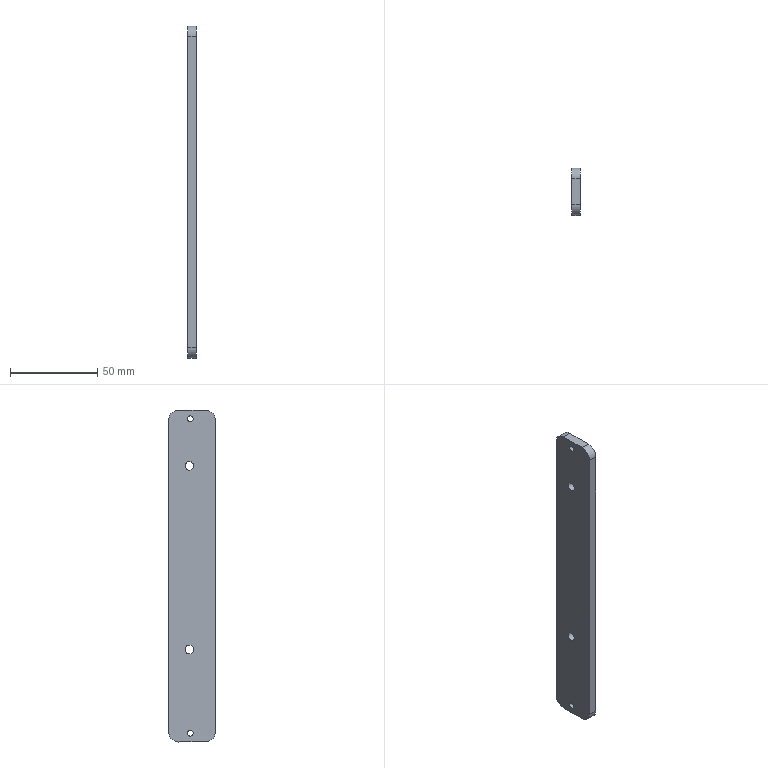CAM job | NX | 3+2 milling, drilling | part box 5 x 27 x 190 mm | stock box 8 x 32 x 195 mm
Tools:
number,name,description,diameter,corner_radius,flute_length,length,flutes
9,D10,平底铣刀-粗,10.0,0.0,35.0,75.0,2
10,D10-J,平底铣刀-精,10.0,0.0,35.0,75.0,2
1,D80R0.8飞刀,圆鼻刀-粗,80.0,0.8,50.0,75.0,2
1,D80R0.8飞刀-J,圆鼻刀-精,80.0,0.8,50.0,75.0,2
2,D6倒角刀,倒角刀,6.0,0.0,3.0,25.0,2
21,M4X0.7,丝锥,3.3,0.0,35.0,50.0,2
23,M6X1.0,丝锥,5.0,0.0,35.0,50.0,2
15,ZT5,钻头,5.0,0.0,35.0,50.0,2
13,钻头3.3,Twist Drill 3.3 mm,3.3,0.0,35.0,35.008,2
Operations:
program,operation,operation_type,tool,method,geometry_group,spindle_rpm,surface_speed,feed_per_tooth,feed_cut,feed_plunge,cut_length_mm,path_length_mm,cut_time_min,machine_time_min
B,底壁铣飞面一刀开粗_COPY,VolumeBased25DMillingOperation,D80R0.8飞刀,分层开粗-切深K-步距G,W-B,2800.0,703.696,0.5357,3000.0,100.0,1192.776,2109.734,0.3976,0.4893
B,底壁铣飞面一刀精光_COPY,VolumeBased25DMillingOperation,D80R0.8飞刀-J,侧刃精光-切深K-步距G,W-B,4000.0,1005.28,0.125,1000.0,100.0,297.998,333.998,0.298,0.3016
B,钻倒角_3,Operation,D6倒角刀,METHOD,W-B,8000.0,150.796,0.0625,1000.0,0.0,10.4,243.825,0.0104,0.0337
B,铣倒角_2,PlanarMilling,D6倒角刀,METHOD,W-B,8000.0,150.796,0.0375,600.0,100.0,37.911,226.569,0.0632,0.0821
B,C0.3封闭铣廓倒角6X45L_COPY,PlanarMilling,D6倒角刀,爬面_倒角-切深0-步距G,W-B,7000.0,131.0,0.1071,1500.0,100.0,441.331,477.331,0.2942,0.2978
A,顶面,FaceMilling,D80R0.8飞刀,侧刃精光-切深K-步距G,W-A,4000.0,1005.31,0.125,1000.0,100.0,284.0,320.0,0.284,0.2876
A,外形粗_2,VolumeBased25DMillingOperation,D10,METHOD,W-A,8000.0,251.327,0.3125,5000.0,80.0,4103.194,4146.794,0.8206,0.825
A,打点-深0.8,Operation,D6倒角刀,NONE,W-A,8000.0,150.796,0.0312,500.0,90.0,7.2,237.44,0.0144,0.0374
A,通孔-M4螺纹底孔,Operation,钻头3.3,NONE,W-A,3000.0,31.102,0.05,300.0,90.0,23.983,268.969,0.0799,0.1044
A,通孔-M6螺纹底孔,Operation,ZT5,NONE,W-A,2800.0,43.982,0.0625,350.0,90.0,27.004,200.058,0.0772,0.0945
A,仅选体,SurfaceContour,D6倒角刀,METHOD,W-A,8000.0,150.796,0.1875,3000.0,100.0,441.011,476.812,0.147,0.1506
A,钻倒角_1,Operation,D6倒角刀,METHOD,W-A,8000.0,150.796,0.0312,500.0,0.0,10.4,243.825,0.0208,0.0441
A,铣倒角_1,PlanarMilling,D6倒角刀,METHOD,W-A,8000.0,150.796,0.0312,500.0,100.0,39.876,227.341,0.0798,0.0985
A,通孔-攻牙M4,Operation,M4X0.7,METHOD,W-A,600.0,6.22,0.0006,0.7,90.0,18.0,257.003,25.714,25.738
A,通孔-攻牙M6,Operation,M6X1.0,METHOD,W-A,500.0,7.854,0.001,1.0,90.0,19.0,184.049,19.0,19.017
A,外形半精_2,VolumeBased25DMillingOperation,D10-J,METHOD,W-A,8000.0,251.327,0.0625,1000.0,100.0,460.115,509.315,0.4601,0.465